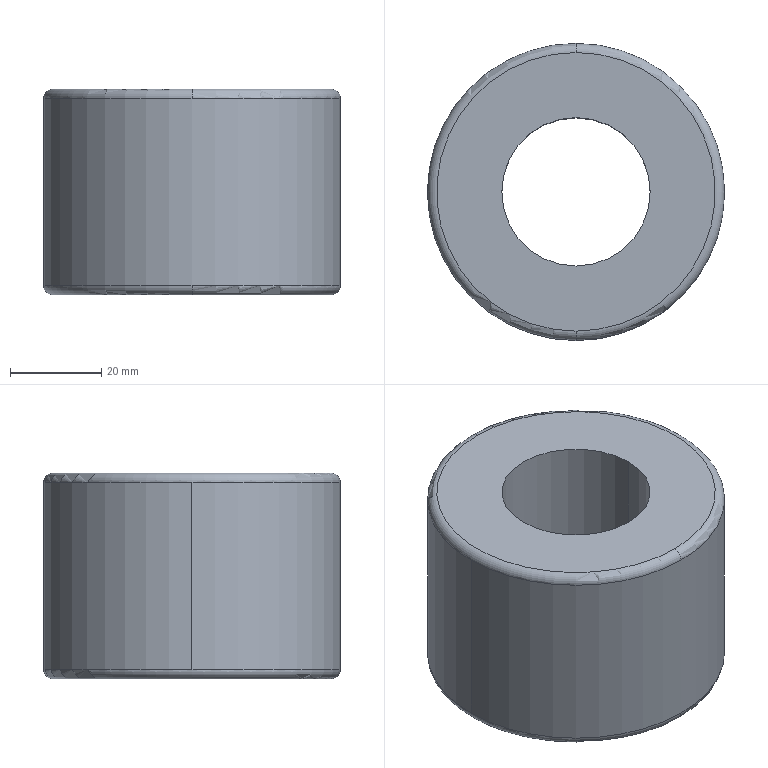Part | SolidWorks | features BaseBody 1 | 1 solid | 10 faces | box 65 x 65 x 45 mm | volume 111647 mm3 | torus 4 | cylinder 4 | plane 2 | commonest cylinder face diameters 32.5 x2 65 x2
STEP:
#1=CARTESIAN_POINT('',(14.,-92.,-20.5));
#2=VERTEX_POINT('',#1);
#3=CARTESIAN_POINT('',(46.5,-59.5,-20.5));
#4=VERTEX_POINT('',#3);
#5=CARTESIAN_POINT('',(14.,-59.5,-20.5));
#6=DIRECTION('',(0.,0.,1.));
#7=DIRECTION('',(1.,0.,0.));
#8=AXIS2_PLACEMENT_3D('',#5,#6,#7);
#9=CIRCLE('',#8,32.5);
#10=EDGE_CURVE('',#2,#4,#9,.T.);
#11=ORIENTED_EDGE('',*,*,#10,.F.);
#12=CARTESIAN_POINT('',(14.,-90.,-22.5));
#13=VERTEX_POINT('',#12);
#14=CARTESIAN_POINT('',(14.,-90.,-20.5));
#15=DIRECTION('',(1.,0.,0.));
#16=DIRECTION('',(0.,1.,0.));
#17=AXIS2_PLACEMENT_3D('',#14,#15,#16);
#18=CIRCLE('',#17,2.);
#19=EDGE_CURVE('',#2,#13,#18,.T.);
#20=ORIENTED_EDGE('',*,*,#19,.T.);
#21=CARTESIAN_POINT('',(14.,-29.,-22.5));
#22=VERTEX_POINT('',#21);
#23=CARTESIAN_POINT('',(14.,-59.5,-22.5));
#24=DIRECTION('',(0.,0.,1.));
#25=DIRECTION('',(-1.,0.,0.));
#26=AXIS2_PLACEMENT_3D('',#23,#24,#25);
#27=CIRCLE('',#26,30.5);
#28=EDGE_CURVE('',#13,#22,#27,.T.);
#29=ORIENTED_EDGE('',*,*,#28,.T.);
#30=CARTESIAN_POINT('',(14.,-27.,-20.5));
#31=VERTEX_POINT('',#30);
#32=CARTESIAN_POINT('',(14.,-29.,-20.5));
#33=DIRECTION('',(-1.,0.,0.));
#34=DIRECTION('',(0.,0.,1.));
#35=AXIS2_PLACEMENT_3D('',#32,#33,#34);
#36=CIRCLE('',#35,2.);
#37=EDGE_CURVE('',#31,#22,#36,.T.);
#38=ORIENTED_EDGE('',*,*,#37,.F.);
#39=CARTESIAN_POINT('',(14.,-59.5,-20.5));
#40=DIRECTION('',(0.,0.,1.));
#41=DIRECTION('',(1.,0.,0.));
#42=AXIS2_PLACEMENT_3D('',#39,#40,#41);
#43=CIRCLE('',#42,32.5);
#44=EDGE_CURVE('',#4,#31,#43,.T.);
#45=ORIENTED_EDGE('',*,*,#44,.F.);
#46=EDGE_LOOP('',(#11,#20,#29,#38,#45));
#47=FACE_OUTER_BOUND('',#46,.T.);
#48=CARTESIAN_POINT('',(14.,-59.5,-20.5));
#49=DIRECTION('',(0.,0.,-1.));
#50=DIRECTION('',(0.,1.,0.));
#51=AXIS2_PLACEMENT_3D('',#48,#49,#50);
#52=TOROIDAL_SURFACE('',#51,30.5,2.);
#53=ADVANCED_FACE('',(#47),#52,.T.);
#54=CARTESIAN_POINT('',(14.,-29.,22.5));
#55=VERTEX_POINT('',#54);
#56=CARTESIAN_POINT('',(14.,-90.,22.5));
#57=VERTEX_POINT('',#56);
#58=CARTESIAN_POINT('',(14.,-59.5,22.5));
#59=DIRECTION('',(0.,0.,-1.));
#60=DIRECTION('',(1.,0.,0.));
#61=AXIS2_PLACEMENT_3D('',#58,#59,#60);
#62=CIRCLE('',#61,30.5);
#63=EDGE_CURVE('',#55,#57,#62,.T.);
#64=ORIENTED_EDGE('',*,*,#63,.T.);
#65=CARTESIAN_POINT('',(14.,-92.,20.5));
#66=VERTEX_POINT('',#65);
#67=CARTESIAN_POINT('',(14.,-90.,20.5));
#68=DIRECTION('',(1.,0.,0.));
#69=DIRECTION('',(0.,1.,0.));
#70=AXIS2_PLACEMENT_3D('',#67,#68,#69);
#71=CIRCLE('',#70,2.);
#72=EDGE_CURVE('',#57,#66,#71,.T.);
#73=ORIENTED_EDGE('',*,*,#72,.T.);
#74=CARTESIAN_POINT('',(46.5,-59.5,20.5));
#75=VERTEX_POINT('',#74);
#76=CARTESIAN_POINT('',(14.,-59.5,20.5));
#77=DIRECTION('',(0.,0.,-1.));
#78=DIRECTION('',(1.,0.,0.));
#79=AXIS2_PLACEMENT_3D('',#76,#77,#78);
#80=CIRCLE('',#79,32.5);
#81=EDGE_CURVE('',#75,#66,#80,.T.);
#82=ORIENTED_EDGE('',*,*,#81,.F.);
#83=CARTESIAN_POINT('',(14.,-27.,20.5));
#84=VERTEX_POINT('',#83);
#85=CARTESIAN_POINT('',(14.,-59.5,20.5));
#86=DIRECTION('',(0.,0.,-1.));
#87=DIRECTION('',(1.,0.,0.));
#88=AXIS2_PLACEMENT_3D('',#85,#86,#87);
#89=CIRCLE('',#88,32.5);
#90=EDGE_CURVE('',#84,#75,#89,.T.);
#91=ORIENTED_EDGE('',*,*,#90,.F.);
#92=CARTESIAN_POINT('',(14.,-29.,20.5));
#93=DIRECTION('',(-1.,0.,0.));
#94=DIRECTION('',(0.,0.,1.));
#95=AXIS2_PLACEMENT_3D('',#92,#93,#94);
#96=CIRCLE('',#95,2.);
#97=EDGE_CURVE('',#55,#84,#96,.T.);
#98=ORIENTED_EDGE('',*,*,#97,.F.);
#99=EDGE_LOOP('',(#64,#73,#82,#91,#98));
#100=FACE_OUTER_BOUND('',#99,.T.);
#101=CARTESIAN_POINT('',(14.,-59.5,20.5));
#102=DIRECTION('',(0.,0.,-1.));
#103=DIRECTION('',(0.,1.,0.));
#104=AXIS2_PLACEMENT_3D('',#101,#102,#103);
#105=TOROIDAL_SURFACE('',#104,30.5,2.);
#106=ADVANCED_FACE('',(#100),#105,.T.);
#107=ORIENTED_EDGE('',*,*,#44,.T.);
#108=CARTESIAN_POINT('',(-18.5,-59.5,-20.5));
#109=VERTEX_POINT('',#108);
#110=CARTESIAN_POINT('',(14.,-59.5,-20.5));
#111=DIRECTION('',(0.,0.,1.));
#112=DIRECTION('',(1.,0.,0.));
#113=AXIS2_PLACEMENT_3D('',#110,#111,#112);
#114=CIRCLE('',#113,32.5);
#115=EDGE_CURVE('',#31,#109,#114,.T.);
#116=ORIENTED_EDGE('',*,*,#115,.T.);
#117=CARTESIAN_POINT('',(-18.5,-59.5,20.5));
#118=VERTEX_POINT('',#117);
#119=CARTESIAN_POINT('',(-18.5,-59.5,0.));
#120=DIRECTION('',(0.,0.,1.));
#121=VECTOR('',#120,1000.);
#122=LINE('',#119,#121);
#123=EDGE_CURVE('',#109,#118,#122,.T.);
#124=ORIENTED_EDGE('',*,*,#123,.T.);
#125=CARTESIAN_POINT('',(14.,-59.5,20.5));
#126=DIRECTION('',(0.,0.,-1.));
#127=DIRECTION('',(1.,0.,0.));
#128=AXIS2_PLACEMENT_3D('',#125,#126,#127);
#129=CIRCLE('',#128,32.5);
#130=EDGE_CURVE('',#118,#84,#129,.T.);
#131=ORIENTED_EDGE('',*,*,#130,.T.);
#132=ORIENTED_EDGE('',*,*,#90,.T.);
#133=CARTESIAN_POINT('',(46.5,-59.5,0.));
#134=DIRECTION('',(0.,0.,1.));
#135=VECTOR('',#134,1000.);
#136=LINE('',#133,#135);
#137=EDGE_CURVE('',#4,#75,#136,.T.);
#138=ORIENTED_EDGE('',*,*,#137,.F.);
#139=EDGE_LOOP('',(#107,#116,#124,#131,#132,#138));
#140=FACE_OUTER_BOUND('',#139,.T.);
#141=CARTESIAN_POINT('',(14.,-59.5,0.));
#142=DIRECTION('',(0.,0.,1.));
#143=DIRECTION('',(1.,0.,0.));
#144=AXIS2_PLACEMENT_3D('',#141,#142,#143);
#145=CYLINDRICAL_SURFACE('',#144,32.5);
#146=ADVANCED_FACE('',(#140),#145,.T.);
#147=CARTESIAN_POINT('',(-2.25,-59.5,-22.5));
#148=VERTEX_POINT('',#147);
#149=CARTESIAN_POINT('',(30.25,-59.5,-22.5));
#150=VERTEX_POINT('',#149);
#151=CARTESIAN_POINT('',(14.,-59.5,-22.5));
#152=DIRECTION('',(0.,0.,1.));
#153=DIRECTION('',(1.,0.,0.));
#154=AXIS2_PLACEMENT_3D('',#151,#152,#153);
#155=CIRCLE('',#154,16.25);
#156=EDGE_CURVE('',#148,#150,#155,.T.);
#157=ORIENTED_EDGE('',*,*,#156,.F.);
#158=CARTESIAN_POINT('',(-2.25,-59.5,22.5));
#159=VERTEX_POINT('',#158);
#160=CARTESIAN_POINT('',(-2.25,-59.5,0.));
#161=DIRECTION('',(0.,0.,1.));
#162=VECTOR('',#161,1000.);
#163=LINE('',#160,#162);
#164=EDGE_CURVE('',#148,#159,#163,.T.);
#165=ORIENTED_EDGE('',*,*,#164,.T.);
#166=CARTESIAN_POINT('',(30.25,-59.5,22.5));
#167=VERTEX_POINT('',#166);
#168=CARTESIAN_POINT('',(14.,-59.5,22.5));
#169=DIRECTION('',(0.,0.,-1.));
#170=DIRECTION('',(1.,0.,0.));
#171=AXIS2_PLACEMENT_3D('',#168,#169,#170);
#172=CIRCLE('',#171,16.25);
#173=EDGE_CURVE('',#167,#159,#172,.T.);
#174=ORIENTED_EDGE('',*,*,#173,.F.);
#175=CARTESIAN_POINT('',(30.25,-59.5,0.));
#176=DIRECTION('',(0.,0.,1.));
#177=VECTOR('',#176,1000.);
#178=LINE('',#175,#177);
#179=EDGE_CURVE('',#150,#167,#178,.T.);
#180=ORIENTED_EDGE('',*,*,#179,.F.);
#181=EDGE_LOOP('',(#157,#165,#174,#180));
#182=FACE_OUTER_BOUND('',#181,.T.);
#183=CARTESIAN_POINT('',(14.,-59.5,0.));
#184=DIRECTION('',(0.,0.,1.));
#185=DIRECTION('',(1.,0.,0.));
#186=AXIS2_PLACEMENT_3D('',#183,#184,#185);
#187=CYLINDRICAL_SURFACE('',#186,16.25);
#188=ADVANCED_FACE('',(#182),#187,.F.);
#189=ORIENTED_EDGE('',*,*,#173,.T.);
#190=CARTESIAN_POINT('',(14.,-59.5,22.5));
#191=DIRECTION('',(0.,0.,-1.));
#192=DIRECTION('',(1.,0.,0.));
#193=AXIS2_PLACEMENT_3D('',#190,#191,#192);
#194=CIRCLE('',#193,16.25);
#195=EDGE_CURVE('',#159,#167,#194,.T.);
#196=ORIENTED_EDGE('',*,*,#195,.T.);
#197=EDGE_LOOP('',(#189,#196));
#198=FACE_BOUND('',#197,.T.);
#199=ORIENTED_EDGE('',*,*,#63,.F.);
#200=CARTESIAN_POINT('',(14.,-59.5,22.5));
#201=DIRECTION('',(0.,0.,-1.));
#202=DIRECTION('',(1.,0.,0.));
#203=AXIS2_PLACEMENT_3D('',#200,#201,#202);
#204=CIRCLE('',#203,30.5);
#205=EDGE_CURVE('',#57,#55,#204,.T.);
#206=ORIENTED_EDGE('',*,*,#205,.F.);
#207=EDGE_LOOP('',(#199,#206));
#208=FACE_OUTER_BOUND('',#207,.T.);
#209=CARTESIAN_POINT('',(14.,-36.125,22.5));
#210=DIRECTION('',(0.,0.,1.));
#211=DIRECTION('',(1.,0.,0.));
#212=AXIS2_PLACEMENT_3D('',#209,#210,#211);
#213=PLANE('',#212);
#214=ADVANCED_FACE('',(#198,#208),#213,.T.);
#215=CARTESIAN_POINT('',(14.,-59.5,-22.5));
#216=DIRECTION('',(0.,0.,1.));
#217=DIRECTION('',(1.,0.,0.));
#218=AXIS2_PLACEMENT_3D('',#215,#216,#217);
#219=CIRCLE('',#218,16.25);
#220=EDGE_CURVE('',#150,#148,#219,.T.);
#221=ORIENTED_EDGE('',*,*,#220,.T.);
#222=ORIENTED_EDGE('',*,*,#156,.T.);
#223=EDGE_LOOP('',(#221,#222));
#224=FACE_BOUND('',#223,.T.);
#225=CARTESIAN_POINT('',(14.,-59.5,-22.5));
#226=DIRECTION('',(0.,0.,1.));
#227=DIRECTION('',(-1.,0.,0.));
#228=AXIS2_PLACEMENT_3D('',#225,#226,#227);
#229=CIRCLE('',#228,30.5);
#230=EDGE_CURVE('',#22,#13,#229,.T.);
#231=ORIENTED_EDGE('',*,*,#230,.F.);
#232=ORIENTED_EDGE('',*,*,#28,.F.);
#233=EDGE_LOOP('',(#231,#232));
#234=FACE_OUTER_BOUND('',#233,.T.);
#235=CARTESIAN_POINT('',(14.,-36.125,-22.5));
#236=DIRECTION('',(0.,0.,-1.));
#237=DIRECTION('',(0.,-1.,0.));
#238=AXIS2_PLACEMENT_3D('',#235,#236,#237);
#239=PLANE('',#238);
#240=ADVANCED_FACE('',(#224,#234),#239,.T.);
#241=ORIENTED_EDGE('',*,*,#164,.F.);
#242=ORIENTED_EDGE('',*,*,#220,.F.);
#243=ORIENTED_EDGE('',*,*,#179,.T.);
#244=ORIENTED_EDGE('',*,*,#195,.F.);
#245=EDGE_LOOP('',(#241,#242,#243,#244));
#246=FACE_OUTER_BOUND('',#245,.T.);
#247=CARTESIAN_POINT('',(14.,-59.5,0.));
#248=DIRECTION('',(0.,0.,1.));
#249=DIRECTION('',(1.,0.,0.));
#250=AXIS2_PLACEMENT_3D('',#247,#248,#249);
#251=CYLINDRICAL_SURFACE('',#250,16.25);
#252=ADVANCED_FACE('',(#246),#251,.F.);
#253=ORIENTED_EDGE('',*,*,#123,.F.);
#254=CARTESIAN_POINT('',(14.,-59.5,-20.5));
#255=DIRECTION('',(0.,0.,1.));
#256=DIRECTION('',(1.,0.,0.));
#257=AXIS2_PLACEMENT_3D('',#254,#255,#256);
#258=CIRCLE('',#257,32.5);
#259=EDGE_CURVE('',#109,#2,#258,.T.);
#260=ORIENTED_EDGE('',*,*,#259,.T.);
#261=ORIENTED_EDGE('',*,*,#10,.T.);
#262=ORIENTED_EDGE('',*,*,#137,.T.);
#263=ORIENTED_EDGE('',*,*,#81,.T.);
#264=CARTESIAN_POINT('',(14.,-59.5,20.5));
#265=DIRECTION('',(0.,0.,-1.));
#266=DIRECTION('',(1.,0.,0.));
#267=AXIS2_PLACEMENT_3D('',#264,#265,#266);
#268=CIRCLE('',#267,32.5);
#269=EDGE_CURVE('',#66,#118,#268,.T.);
#270=ORIENTED_EDGE('',*,*,#269,.T.);
#271=EDGE_LOOP('',(#253,#260,#261,#262,#263,#270));
#272=FACE_OUTER_BOUND('',#271,.T.);
#273=CARTESIAN_POINT('',(14.,-59.5,0.));
#274=DIRECTION('',(0.,0.,1.));
#275=DIRECTION('',(1.,0.,0.));
#276=AXIS2_PLACEMENT_3D('',#273,#274,#275);
#277=CYLINDRICAL_SURFACE('',#276,32.5);
#278=ADVANCED_FACE('',(#272),#277,.T.);
#279=ORIENTED_EDGE('',*,*,#72,.F.);
#280=ORIENTED_EDGE('',*,*,#205,.T.);
#281=ORIENTED_EDGE('',*,*,#97,.T.);
#282=ORIENTED_EDGE('',*,*,#130,.F.);
#283=ORIENTED_EDGE('',*,*,#269,.F.);
#284=EDGE_LOOP('',(#279,#280,#281,#282,#283));
#285=FACE_OUTER_BOUND('',#284,.T.);
#286=CARTESIAN_POINT('',(14.,-59.5,20.5));
#287=DIRECTION('',(0.,0.,-1.));
#288=DIRECTION('',(0.,1.,0.));
#289=AXIS2_PLACEMENT_3D('',#286,#287,#288);
#290=TOROIDAL_SURFACE('',#289,30.5,2.);
#291=ADVANCED_FACE('',(#285),#290,.T.);
#292=ORIENTED_EDGE('',*,*,#19,.F.);
#293=ORIENTED_EDGE('',*,*,#259,.F.);
#294=ORIENTED_EDGE('',*,*,#115,.F.);
#295=ORIENTED_EDGE('',*,*,#37,.T.);
#296=ORIENTED_EDGE('',*,*,#230,.T.);
#297=EDGE_LOOP('',(#292,#293,#294,#295,#296));
#298=FACE_OUTER_BOUND('',#297,.T.);
#299=CARTESIAN_POINT('',(14.,-59.5,-20.5));
#300=DIRECTION('',(0.,0.,-1.));
#301=DIRECTION('',(0.,1.,0.));
#302=AXIS2_PLACEMENT_3D('',#299,#300,#301);
#303=TOROIDAL_SURFACE('',#302,30.5,2.);
#304=ADVANCED_FACE('',(#298),#303,.T.);
#305=CLOSED_SHELL('',(#53,#106,#146,#188,#214,#240,#252,#278,#291,#304));
#306=MANIFOLD_SOLID_BREP('',#305);
#307=CARTESIAN_POINT('',(0.,0.,0.));
#308=DIRECTION('',(0.,0.,1.));
#309=DIRECTION('',(1.,0.,0.));
#310=AXIS2_PLACEMENT_3D('',#307,#308,#309);
#311=(LENGTH_UNIT()NAMED_UNIT(*)SI_UNIT(.MILLI.,.METRE.));
#312=UNCERTAINTY_MEASURE_WITH_UNIT(LENGTH_MEASURE(0.00001),#311,'','');
#313=(NAMED_UNIT(*)PLANE_ANGLE_UNIT()SI_UNIT($,.RADIAN.));
#314=(NAMED_UNIT(*)SI_UNIT($,.STERADIAN.)SOLID_ANGLE_UNIT());
#315=(GEOMETRIC_REPRESENTATION_CONTEXT(3)GLOBAL_UNCERTAINTY_ASSIGNED_CONTEXT((#312))GLOBAL_UNIT_ASSIGNED_CONTEXT((#311,#313,#314))REPRESENTATION_CONTEXT('',''));
#316=ADVANCED_BREP_SHAPE_REPRESENTATION('',(#306,#310),#315);